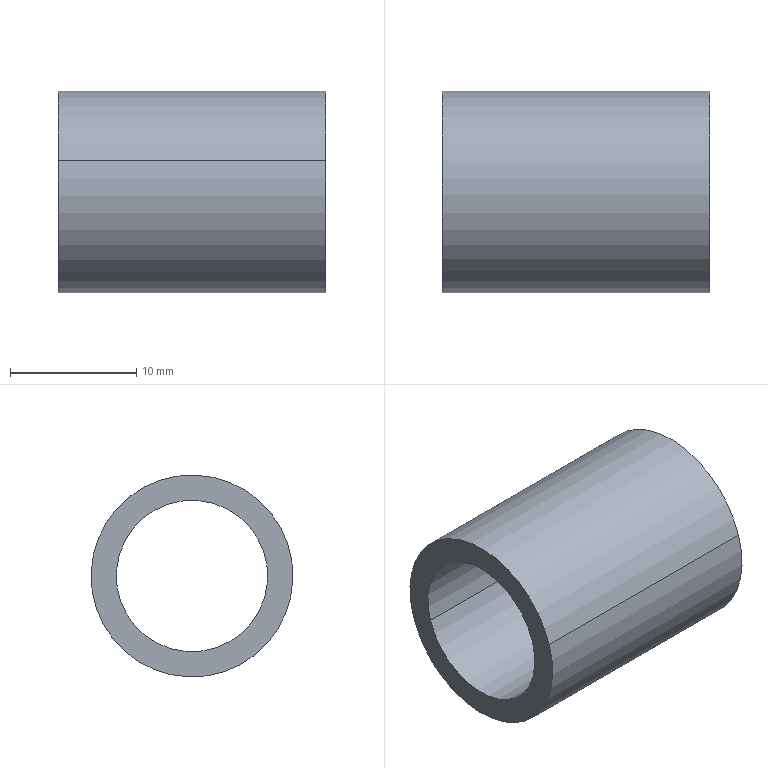Part | STEP file | Completa.sldasm-Part-4_Valor predeterminado | 1 solid | 6 faces | box 21.228 x 16 x 16 mm | volume 1867 mm3 | cylinder 4 | plane 2 | commonest cylinder face diameters 12 x2 16 x2
STEP:
#1=CARTESIAN_POINT('',(0.,0.,0.));
#2=DIRECTION('',(0.,0.,1.));
#3=DIRECTION('',(1.,0.,0.));
#4=AXIS2_PLACEMENT_3D('',#1,#2,#3);
#5=CARTESIAN_POINT('',(-204.167,20.156,-33.743));
#6=VERTEX_POINT('',#5);
#7=CARTESIAN_POINT('',(-225.395,20.156,-33.743));
#8=VERTEX_POINT('',#7);
#9=CARTESIAN_POINT('',(-204.167,20.156,-33.743));
#10=DIRECTION('',(-1.,0.,0.));
#11=VECTOR('',#10,1.);
#12=LINE('',#9,#11);
#13=CARTESIAN_POINT('',(-204.167,25.863,-35.597));
#14=DIRECTION('',(-1.,0.,0.));
#15=DIRECTION('',(0.,-0.9511,0.309));
#16=AXIS2_PLACEMENT_3D('',#13,#14,#15);
#17=CYLINDRICAL_SURFACE('',#16,6.);
#18=CARTESIAN_POINT('',(6.283,0.));
#19=DIRECTION('',(0.,1.));
#20=VECTOR('',#19,1.);
#21=LINE('',#18,#20);
#22=(GEOMETRIC_REPRESENTATION_CONTEXT(2)PARAMETRIC_REPRESENTATION_CONTEXT()REPRESENTATION_CONTEXT('',''));
#23=DEFINITIONAL_REPRESENTATION('',(#21),#22);
#24=PCURVE('',#17,#23);
#25=CARTESIAN_POINT('',(-204.167,25.863,-35.597));
#26=DIRECTION('',(-1.,0.,0.));
#27=DIRECTION('',(0.,-0.9511,0.309));
#28=AXIS2_PLACEMENT_3D('',#25,#26,#27);
#29=CYLINDRICAL_SURFACE('',#28,6.);
#30=CARTESIAN_POINT('',(0.,0.));
#31=DIRECTION('',(0.,1.));
#32=VECTOR('',#31,1.);
#33=LINE('',#30,#32);
#34=(GEOMETRIC_REPRESENTATION_CONTEXT(2)PARAMETRIC_REPRESENTATION_CONTEXT()REPRESENTATION_CONTEXT('',''));
#35=DEFINITIONAL_REPRESENTATION('',(#33),#34);
#36=PCURVE('',#29,#35);
#37=SURFACE_CURVE('',#12,(#24,#36),.PCURVE_S1.);
#38=EDGE_CURVE('',#6,#8,#37,.T.);
#39=ORIENTED_EDGE('',*,*,#38,.T.);
#40=CARTESIAN_POINT('',(-225.395,31.569,-37.451));
#41=VERTEX_POINT('',#40);
#42=CARTESIAN_POINT('',(-225.395,25.863,-35.597));
#43=DIRECTION('',(-1.,0.,0.));
#44=DIRECTION('',(0.,0.9511,-0.309));
#45=AXIS2_PLACEMENT_3D('',#42,#43,#44);
#46=CIRCLE('',#45,6.);
#47=CARTESIAN_POINT('',(3.142,21.228));
#48=DIRECTION('',(1.,0.));
#49=VECTOR('',#48,1.);
#50=LINE('',#47,#49);
#51=(GEOMETRIC_REPRESENTATION_CONTEXT(2)PARAMETRIC_REPRESENTATION_CONTEXT()REPRESENTATION_CONTEXT('',''));
#52=DEFINITIONAL_REPRESENTATION('',(#50),#51);
#53=PCURVE('',#17,#52);
#54=CARTESIAN_POINT('',(-225.395,-10.072,-30.999));
#55=DIRECTION('',(1.,0.,0.));
#56=DIRECTION('',(0.,0.9511,-0.309));
#57=AXIS2_PLACEMENT_3D('',#54,#55,#56);
#58=PLANE('',#57);
#59=CARTESIAN_POINT('',(41.597,6.731));
#60=CARTESIAN_POINT('',(41.597,-3.661));
#61=CARTESIAN_POINT('',(32.597,1.535));
#62=CARTESIAN_POINT('',(23.597,6.731));
#63=CARTESIAN_POINT('',(32.597,11.927));
#64=CARTESIAN_POINT('',(41.597,17.124));
#65=CARTESIAN_POINT('',(41.597,6.731));
#66=(BOUNDED_CURVE()B_SPLINE_CURVE(2,(#59,#60,#61,#62,#63,#64,#65),.UNSPECIFIED.,.T.,.F.)B_SPLINE_CURVE_WITH_KNOTS((1,2,2,2,2,1),(-2.094,0.,2.094,4.189,6.283,8.378),.UNSPECIFIED.)CURVE()GEOMETRIC_REPRESENTATION_ITEM()RATIONAL_B_SPLINE_CURVE((1.,0.5,1.,0.5,1.,0.5,1.))REPRESENTATION_ITEM(''));
#67=(GEOMETRIC_REPRESENTATION_CONTEXT(2)PARAMETRIC_REPRESENTATION_CONTEXT()REPRESENTATION_CONTEXT('',''));
#68=DEFINITIONAL_REPRESENTATION('',(#66),#67);
#69=PCURVE('',#58,#68);
#70=SURFACE_CURVE('',#46,(#53,#69),.PCURVE_S1.);
#71=EDGE_CURVE('',#41,#8,#70,.T.);
#72=ORIENTED_EDGE('',*,*,#71,.F.);
#73=CARTESIAN_POINT('',(-204.167,31.569,-37.451));
#74=VERTEX_POINT('',#73);
#75=CARTESIAN_POINT('',(-204.167,31.569,-37.451));
#76=DIRECTION('',(-1.,0.,0.));
#77=VECTOR('',#76,1.);
#78=LINE('',#75,#77);
#79=CARTESIAN_POINT('',(3.142,0.));
#80=DIRECTION('',(0.,1.));
#81=VECTOR('',#80,1.);
#82=LINE('',#79,#81);
#83=(GEOMETRIC_REPRESENTATION_CONTEXT(2)PARAMETRIC_REPRESENTATION_CONTEXT()REPRESENTATION_CONTEXT('',''));
#84=DEFINITIONAL_REPRESENTATION('',(#82),#83);
#85=PCURVE('',#17,#84);
#86=CARTESIAN_POINT('',(3.142,0.));
#87=DIRECTION('',(0.,1.));
#88=VECTOR('',#87,1.);
#89=LINE('',#86,#88);
#90=(GEOMETRIC_REPRESENTATION_CONTEXT(2)PARAMETRIC_REPRESENTATION_CONTEXT()REPRESENTATION_CONTEXT('',''));
#91=DEFINITIONAL_REPRESENTATION('',(#89),#90);
#92=PCURVE('',#29,#91);
#93=SURFACE_CURVE('',#78,(#85,#92),.PCURVE_S1.);
#94=EDGE_CURVE('',#74,#41,#93,.T.);
#95=ORIENTED_EDGE('',*,*,#94,.F.);
#96=CARTESIAN_POINT('',(-204.167,25.863,-35.597));
#97=DIRECTION('',(-1.,0.,0.));
#98=DIRECTION('',(0.,-0.9511,0.309));
#99=AXIS2_PLACEMENT_3D('',#96,#97,#98);
#100=CIRCLE('',#99,6.);
#101=CARTESIAN_POINT('',(0.,0.));
#102=DIRECTION('',(1.,0.));
#103=VECTOR('',#102,1.);
#104=LINE('',#101,#103);
#105=(GEOMETRIC_REPRESENTATION_CONTEXT(2)PARAMETRIC_REPRESENTATION_CONTEXT()REPRESENTATION_CONTEXT('',''));
#106=DEFINITIONAL_REPRESENTATION('',(#104),#105);
#107=PCURVE('',#17,#106);
#108=CARTESIAN_POINT('',(-204.167,25.863,-35.597));
#109=DIRECTION('',(1.,0.,0.));
#110=DIRECTION('',(0.,0.9511,-0.309));
#111=AXIS2_PLACEMENT_3D('',#108,#109,#110);
#112=PLANE('',#111);
#113=CARTESIAN_POINT('',(-6.,0.));
#114=CARTESIAN_POINT('',(-6.,10.392));
#115=CARTESIAN_POINT('',(3.,5.196));
#116=CARTESIAN_POINT('',(12.,0.));
#117=CARTESIAN_POINT('',(3.,-5.196));
#118=CARTESIAN_POINT('',(-6.,-10.392));
#119=CARTESIAN_POINT('',(-6.,0.));
#120=(BOUNDED_CURVE()B_SPLINE_CURVE(2,(#113,#114,#115,#116,#117,#118,#119),.UNSPECIFIED.,.T.,.F.)B_SPLINE_CURVE_WITH_KNOTS((1,2,2,2,2,1),(-2.094,0.,2.094,4.189,6.283,8.378),.UNSPECIFIED.)CURVE()GEOMETRIC_REPRESENTATION_ITEM()RATIONAL_B_SPLINE_CURVE((1.,0.5,1.,0.5,1.,0.5,1.))REPRESENTATION_ITEM(''));
#121=(GEOMETRIC_REPRESENTATION_CONTEXT(2)PARAMETRIC_REPRESENTATION_CONTEXT()REPRESENTATION_CONTEXT('',''));
#122=DEFINITIONAL_REPRESENTATION('',(#120),#121);
#123=PCURVE('',#112,#122);
#124=SURFACE_CURVE('',#100,(#107,#123),.PCURVE_S1.);
#125=EDGE_CURVE('',#74,#6,#124,.T.);
#126=ORIENTED_EDGE('',*,*,#125,.T.);
#127=EDGE_LOOP('',(#39,#72,#95,#126));
#128=FACE_BOUND('',#127,.F.);
#129=ADVANCED_FACE('',(#128),#17,.F.);
#130=CARTESIAN_POINT('',(-204.167,18.254,-33.125));
#131=VERTEX_POINT('',#130);
#132=CARTESIAN_POINT('',(-204.167,33.471,-38.069));
#133=VERTEX_POINT('',#132);
#134=CARTESIAN_POINT('',(-204.167,25.863,-35.597));
#135=DIRECTION('',(-1.,0.,0.));
#136=DIRECTION('',(0.,-0.9511,0.309));
#137=AXIS2_PLACEMENT_3D('',#134,#135,#136);
#138=CIRCLE('',#137,8.);
#139=CARTESIAN_POINT('',(-204.167,25.863,-35.597));
#140=DIRECTION('',(-1.,0.,0.));
#141=DIRECTION('',(0.,-0.9511,0.309));
#142=AXIS2_PLACEMENT_3D('',#139,#140,#141);
#143=CYLINDRICAL_SURFACE('',#142,8.);
#144=CARTESIAN_POINT('',(0.,0.));
#145=DIRECTION('',(1.,0.));
#146=VECTOR('',#145,1.);
#147=LINE('',#144,#146);
#148=(GEOMETRIC_REPRESENTATION_CONTEXT(2)PARAMETRIC_REPRESENTATION_CONTEXT()REPRESENTATION_CONTEXT('',''));
#149=DEFINITIONAL_REPRESENTATION('',(#147),#148);
#150=PCURVE('',#143,#149);
#151=CARTESIAN_POINT('',(-8.,0.));
#152=CARTESIAN_POINT('',(-8.,13.856));
#153=CARTESIAN_POINT('',(4.,6.928));
#154=CARTESIAN_POINT('',(16.,0.));
#155=CARTESIAN_POINT('',(4.,-6.928));
#156=CARTESIAN_POINT('',(-8.,-13.856));
#157=CARTESIAN_POINT('',(-8.,0.));
#158=(BOUNDED_CURVE()B_SPLINE_CURVE(2,(#151,#152,#153,#154,#155,#156,#157),.UNSPECIFIED.,.T.,.F.)B_SPLINE_CURVE_WITH_KNOTS((1,2,2,2,2,1),(-2.094,0.,2.094,4.189,6.283,8.378),.UNSPECIFIED.)CURVE()GEOMETRIC_REPRESENTATION_ITEM()RATIONAL_B_SPLINE_CURVE((1.,0.5,1.,0.5,1.,0.5,1.))REPRESENTATION_ITEM(''));
#159=(GEOMETRIC_REPRESENTATION_CONTEXT(2)PARAMETRIC_REPRESENTATION_CONTEXT()REPRESENTATION_CONTEXT('',''));
#160=DEFINITIONAL_REPRESENTATION('',(#158),#159);
#161=PCURVE('',#112,#160);
#162=SURFACE_CURVE('',#138,(#150,#161),.PCURVE_S1.);
#163=EDGE_CURVE('',#131,#133,#162,.T.);
#164=ORIENTED_EDGE('',*,*,#163,.T.);
#165=CARTESIAN_POINT('',(-225.395,33.471,-38.069));
#166=VERTEX_POINT('',#165);
#167=CARTESIAN_POINT('',(-204.167,33.471,-38.069));
#168=DIRECTION('',(-1.,0.,0.));
#169=VECTOR('',#168,1.);
#170=LINE('',#167,#169);
#171=CARTESIAN_POINT('',(3.142,0.));
#172=DIRECTION('',(0.,1.));
#173=VECTOR('',#172,1.);
#174=LINE('',#171,#173);
#175=(GEOMETRIC_REPRESENTATION_CONTEXT(2)PARAMETRIC_REPRESENTATION_CONTEXT()REPRESENTATION_CONTEXT('',''));
#176=DEFINITIONAL_REPRESENTATION('',(#174),#175);
#177=PCURVE('',#143,#176);
#178=CARTESIAN_POINT('',(-204.167,25.863,-35.597));
#179=DIRECTION('',(-1.,0.,0.));
#180=DIRECTION('',(0.,-0.9511,0.309));
#181=AXIS2_PLACEMENT_3D('',#178,#179,#180);
#182=CYLINDRICAL_SURFACE('',#181,8.);
#183=CARTESIAN_POINT('',(3.142,0.));
#184=DIRECTION('',(0.,1.));
#185=VECTOR('',#184,1.);
#186=LINE('',#183,#185);
#187=(GEOMETRIC_REPRESENTATION_CONTEXT(2)PARAMETRIC_REPRESENTATION_CONTEXT()REPRESENTATION_CONTEXT('',''));
#188=DEFINITIONAL_REPRESENTATION('',(#186),#187);
#189=PCURVE('',#182,#188);
#190=SURFACE_CURVE('',#170,(#177,#189),.PCURVE_S1.);
#191=EDGE_CURVE('',#133,#166,#190,.T.);
#192=ORIENTED_EDGE('',*,*,#191,.T.);
#193=CARTESIAN_POINT('',(-225.395,18.254,-33.125));
#194=VERTEX_POINT('',#193);
#195=CARTESIAN_POINT('',(-225.395,25.863,-35.597));
#196=DIRECTION('',(-1.,0.,0.));
#197=DIRECTION('',(0.,0.9511,-0.309));
#198=AXIS2_PLACEMENT_3D('',#195,#196,#197);
#199=CIRCLE('',#198,8.);
#200=CARTESIAN_POINT('',(-3.142,21.228));
#201=DIRECTION('',(1.,0.));
#202=VECTOR('',#201,1.);
#203=LINE('',#200,#202);
#204=(GEOMETRIC_REPRESENTATION_CONTEXT(2)PARAMETRIC_REPRESENTATION_CONTEXT()REPRESENTATION_CONTEXT('',''));
#205=DEFINITIONAL_REPRESENTATION('',(#203),#204);
#206=PCURVE('',#143,#205);
#207=CARTESIAN_POINT('',(43.597,6.731));
#208=CARTESIAN_POINT('',(43.597,-7.125));
#209=CARTESIAN_POINT('',(31.597,-0.1969));
#210=CARTESIAN_POINT('',(19.597,6.731));
#211=CARTESIAN_POINT('',(31.597,13.659));
#212=CARTESIAN_POINT('',(43.597,20.588));
#213=CARTESIAN_POINT('',(43.597,6.731));
#214=(BOUNDED_CURVE()B_SPLINE_CURVE(2,(#207,#208,#209,#210,#211,#212,#213),.UNSPECIFIED.,.T.,.F.)B_SPLINE_CURVE_WITH_KNOTS((1,2,2,2,2,1),(-2.094,0.,2.094,4.189,6.283,8.378),.UNSPECIFIED.)CURVE()GEOMETRIC_REPRESENTATION_ITEM()RATIONAL_B_SPLINE_CURVE((1.,0.5,1.,0.5,1.,0.5,1.))REPRESENTATION_ITEM(''));
#215=(GEOMETRIC_REPRESENTATION_CONTEXT(2)PARAMETRIC_REPRESENTATION_CONTEXT()REPRESENTATION_CONTEXT('',''));
#216=DEFINITIONAL_REPRESENTATION('',(#214),#215);
#217=PCURVE('',#58,#216);
#218=SURFACE_CURVE('',#199,(#206,#217),.PCURVE_S1.);
#219=EDGE_CURVE('',#194,#166,#218,.T.);
#220=ORIENTED_EDGE('',*,*,#219,.F.);
#221=CARTESIAN_POINT('',(-204.167,18.254,-33.125));
#222=DIRECTION('',(-1.,0.,0.));
#223=VECTOR('',#222,1.);
#224=LINE('',#221,#223);
#225=CARTESIAN_POINT('',(0.,0.));
#226=DIRECTION('',(0.,1.));
#227=VECTOR('',#226,1.);
#228=LINE('',#225,#227);
#229=(GEOMETRIC_REPRESENTATION_CONTEXT(2)PARAMETRIC_REPRESENTATION_CONTEXT()REPRESENTATION_CONTEXT('',''));
#230=DEFINITIONAL_REPRESENTATION('',(#228),#229);
#231=PCURVE('',#143,#230);
#232=CARTESIAN_POINT('',(6.283,0.));
#233=DIRECTION('',(0.,1.));
#234=VECTOR('',#233,1.);
#235=LINE('',#232,#234);
#236=(GEOMETRIC_REPRESENTATION_CONTEXT(2)PARAMETRIC_REPRESENTATION_CONTEXT()REPRESENTATION_CONTEXT('',''));
#237=DEFINITIONAL_REPRESENTATION('',(#235),#236);
#238=PCURVE('',#182,#237);
#239=SURFACE_CURVE('',#224,(#231,#238),.PCURVE_S1.);
#240=EDGE_CURVE('',#131,#194,#239,.T.);
#241=ORIENTED_EDGE('',*,*,#240,.F.);
#242=EDGE_LOOP('',(#164,#192,#220,#241));
#243=FACE_BOUND('',#242,.T.);
#244=ADVANCED_FACE('',(#243),#143,.T.);
#245=ORIENTED_EDGE('',*,*,#191,.F.);
#246=CARTESIAN_POINT('',(-204.167,25.863,-35.597));
#247=DIRECTION('',(-1.,0.,0.));
#248=DIRECTION('',(0.,-0.9511,0.309));
#249=AXIS2_PLACEMENT_3D('',#246,#247,#248);
#250=CIRCLE('',#249,8.);
#251=CARTESIAN_POINT('',(0.,0.));
#252=DIRECTION('',(1.,0.));
#253=VECTOR('',#252,1.);
#254=LINE('',#251,#253);
#255=(GEOMETRIC_REPRESENTATION_CONTEXT(2)PARAMETRIC_REPRESENTATION_CONTEXT()REPRESENTATION_CONTEXT('',''));
#256=DEFINITIONAL_REPRESENTATION('',(#254),#255);
#257=PCURVE('',#182,#256);
#258=CARTESIAN_POINT('',(-8.,0.));
#259=CARTESIAN_POINT('',(-8.,13.856));
#260=CARTESIAN_POINT('',(4.,6.928));
#261=CARTESIAN_POINT('',(16.,0.));
#262=CARTESIAN_POINT('',(4.,-6.928));
#263=CARTESIAN_POINT('',(-8.,-13.856));
#264=CARTESIAN_POINT('',(-8.,0.));
#265=(BOUNDED_CURVE()B_SPLINE_CURVE(2,(#258,#259,#260,#261,#262,#263,#264),.UNSPECIFIED.,.T.,.F.)B_SPLINE_CURVE_WITH_KNOTS((1,2,2,2,2,1),(-2.094,0.,2.094,4.189,6.283,8.378),.UNSPECIFIED.)CURVE()GEOMETRIC_REPRESENTATION_ITEM()RATIONAL_B_SPLINE_CURVE((1.,0.5,1.,0.5,1.,0.5,1.))REPRESENTATION_ITEM(''));
#266=(GEOMETRIC_REPRESENTATION_CONTEXT(2)PARAMETRIC_REPRESENTATION_CONTEXT()REPRESENTATION_CONTEXT('',''));
#267=DEFINITIONAL_REPRESENTATION('',(#265),#266);
#268=PCURVE('',#112,#267);
#269=SURFACE_CURVE('',#250,(#257,#268),.PCURVE_S1.);
#270=EDGE_CURVE('',#133,#131,#269,.T.);
#271=ORIENTED_EDGE('',*,*,#270,.T.);
#272=ORIENTED_EDGE('',*,*,#240,.T.);
#273=CARTESIAN_POINT('',(-225.395,25.863,-35.597));
#274=DIRECTION('',(-1.,0.,0.));
#275=DIRECTION('',(0.,0.9511,-0.309));
#276=AXIS2_PLACEMENT_3D('',#273,#274,#275);
#277=CIRCLE('',#276,8.);
#278=CARTESIAN_POINT('',(3.142,21.228));
#279=DIRECTION('',(1.,0.));
#280=VECTOR('',#279,1.);
#281=LINE('',#278,#280);
#282=(GEOMETRIC_REPRESENTATION_CONTEXT(2)PARAMETRIC_REPRESENTATION_CONTEXT()REPRESENTATION_CONTEXT('',''));
#283=DEFINITIONAL_REPRESENTATION('',(#281),#282);
#284=PCURVE('',#182,#283);
#285=CARTESIAN_POINT('',(43.597,6.731));
#286=CARTESIAN_POINT('',(43.597,-7.125));
#287=CARTESIAN_POINT('',(31.597,-0.1969));
#288=CARTESIAN_POINT('',(19.597,6.731));
#289=CARTESIAN_POINT('',(31.597,13.659));
#290=CARTESIAN_POINT('',(43.597,20.588));
#291=CARTESIAN_POINT('',(43.597,6.731));
#292=(BOUNDED_CURVE()B_SPLINE_CURVE(2,(#285,#286,#287,#288,#289,#290,#291),.UNSPECIFIED.,.T.,.F.)B_SPLINE_CURVE_WITH_KNOTS((1,2,2,2,2,1),(-2.094,0.,2.094,4.189,6.283,8.378),.UNSPECIFIED.)CURVE()GEOMETRIC_REPRESENTATION_ITEM()RATIONAL_B_SPLINE_CURVE((1.,0.5,1.,0.5,1.,0.5,1.))REPRESENTATION_ITEM(''));
#293=(GEOMETRIC_REPRESENTATION_CONTEXT(2)PARAMETRIC_REPRESENTATION_CONTEXT()REPRESENTATION_CONTEXT('',''));
#294=DEFINITIONAL_REPRESENTATION('',(#292),#293);
#295=PCURVE('',#58,#294);
#296=SURFACE_CURVE('',#277,(#284,#295),.PCURVE_S1.);
#297=EDGE_CURVE('',#166,#194,#296,.T.);
#298=ORIENTED_EDGE('',*,*,#297,.F.);
#299=EDGE_LOOP('',(#245,#271,#272,#298));
#300=FACE_BOUND('',#299,.T.);
#301=ADVANCED_FACE('',(#300),#182,.T.);
#302=ORIENTED_EDGE('',*,*,#163,.F.);
#303=ORIENTED_EDGE('',*,*,#270,.F.);
#304=EDGE_LOOP('',(#302,#303));
#305=FACE_BOUND('',#304,.T.);
#306=CARTESIAN_POINT('',(-204.167,25.863,-35.597));
#307=DIRECTION('',(-1.,0.,0.));
#308=DIRECTION('',(0.,-0.9511,0.309));
#309=AXIS2_PLACEMENT_3D('',#306,#307,#308);
#310=CIRCLE('',#309,6.);
#311=CARTESIAN_POINT('',(-6.,0.));
#312=CARTESIAN_POINT('',(-6.,10.392));
#313=CARTESIAN_POINT('',(3.,5.196));
#314=CARTESIAN_POINT('',(12.,0.));
#315=CARTESIAN_POINT('',(3.,-5.196));
#316=CARTESIAN_POINT('',(-6.,-10.392));
#317=CARTESIAN_POINT('',(-6.,0.));
#318=(BOUNDED_CURVE()B_SPLINE_CURVE(2,(#311,#312,#313,#314,#315,#316,#317),.UNSPECIFIED.,.T.,.F.)B_SPLINE_CURVE_WITH_KNOTS((1,2,2,2,2,1),(-2.094,0.,2.094,4.189,6.283,8.378),.UNSPECIFIED.)CURVE()GEOMETRIC_REPRESENTATION_ITEM()RATIONAL_B_SPLINE_CURVE((1.,0.5,1.,0.5,1.,0.5,1.))REPRESENTATION_ITEM(''));
#319=(GEOMETRIC_REPRESENTATION_CONTEXT(2)PARAMETRIC_REPRESENTATION_CONTEXT()REPRESENTATION_CONTEXT('',''));
#320=DEFINITIONAL_REPRESENTATION('',(#318),#319);
#321=PCURVE('',#112,#320);
#322=CARTESIAN_POINT('',(0.,0.));
#323=DIRECTION('',(1.,0.));
#324=VECTOR('',#323,1.);
#325=LINE('',#322,#324);
#326=(GEOMETRIC_REPRESENTATION_CONTEXT(2)PARAMETRIC_REPRESENTATION_CONTEXT()REPRESENTATION_CONTEXT('',''));
#327=DEFINITIONAL_REPRESENTATION('',(#325),#326);
#328=PCURVE('',#29,#327);
#329=SURFACE_CURVE('',#310,(#321,#328),.PCURVE_S1.);
#330=EDGE_CURVE('',#6,#74,#329,.T.);
#331=ORIENTED_EDGE('',*,*,#330,.T.);
#332=ORIENTED_EDGE('',*,*,#125,.T.);
#333=EDGE_LOOP('',(#331,#332));
#334=FACE_BOUND('',#333,.T.);
#335=ADVANCED_FACE('',(#305,#334),#112,.T.);
#336=CARTESIAN_POINT('',(-225.395,25.863,-35.597));
#337=DIRECTION('',(-1.,0.,0.));
#338=DIRECTION('',(0.,0.9511,-0.309));
#339=AXIS2_PLACEMENT_3D('',#336,#337,#338);
#340=CIRCLE('',#339,6.);
#341=CARTESIAN_POINT('',(-3.142,21.228));
#342=DIRECTION('',(1.,0.));
#343=VECTOR('',#342,1.);
#344=LINE('',#341,#343);
#345=(GEOMETRIC_REPRESENTATION_CONTEXT(2)PARAMETRIC_REPRESENTATION_CONTEXT()REPRESENTATION_CONTEXT('',''));
#346=DEFINITIONAL_REPRESENTATION('',(#344),#345);
#347=PCURVE('',#29,#346);
#348=CARTESIAN_POINT('',(41.597,6.731));
#349=CARTESIAN_POINT('',(41.597,-3.661));
#350=CARTESIAN_POINT('',(32.597,1.535));
#351=CARTESIAN_POINT('',(23.597,6.731));
#352=CARTESIAN_POINT('',(32.597,11.927));
#353=CARTESIAN_POINT('',(41.597,17.124));
#354=CARTESIAN_POINT('',(41.597,6.731));
#355=(BOUNDED_CURVE()B_SPLINE_CURVE(2,(#348,#349,#350,#351,#352,#353,#354),.UNSPECIFIED.,.T.,.F.)B_SPLINE_CURVE_WITH_KNOTS((1,2,2,2,2,1),(-2.094,0.,2.094,4.189,6.283,8.378),.UNSPECIFIED.)CURVE()GEOMETRIC_REPRESENTATION_ITEM()RATIONAL_B_SPLINE_CURVE((1.,0.5,1.,0.5,1.,0.5,1.))REPRESENTATION_ITEM(''));
#356=(GEOMETRIC_REPRESENTATION_CONTEXT(2)PARAMETRIC_REPRESENTATION_CONTEXT()REPRESENTATION_CONTEXT('',''));
#357=DEFINITIONAL_REPRESENTATION('',(#355),#356);
#358=PCURVE('',#58,#357);
#359=SURFACE_CURVE('',#340,(#347,#358),.PCURVE_S1.);
#360=EDGE_CURVE('',#8,#41,#359,.T.);
#361=ORIENTED_EDGE('',*,*,#360,.F.);
#362=ORIENTED_EDGE('',*,*,#38,.F.);
#363=ORIENTED_EDGE('',*,*,#330,.T.);
#364=ORIENTED_EDGE('',*,*,#94,.T.);
#365=EDGE_LOOP('',(#361,#362,#363,#364));
#366=FACE_BOUND('',#365,.F.);
#367=ADVANCED_FACE('',(#366),#29,.F.);
#368=ORIENTED_EDGE('',*,*,#219,.T.);
#369=ORIENTED_EDGE('',*,*,#297,.T.);
#370=EDGE_LOOP('',(#368,#369));
#371=FACE_BOUND('',#370,.T.);
#372=ORIENTED_EDGE('',*,*,#360,.F.);
#373=ORIENTED_EDGE('',*,*,#71,.F.);
#374=EDGE_LOOP('',(#372,#373));
#375=FACE_BOUND('',#374,.T.);
#376=ADVANCED_FACE('',(#371,#375),#58,.F.);
#377=CLOSED_SHELL('',(#129,#244,#301,#335,#367,#376));
#378=MANIFOLD_SOLID_BREP('',#377);
#379=(LENGTH_UNIT()NAMED_UNIT(*)SI_UNIT(.MILLI.,.METRE.));
#380=UNCERTAINTY_MEASURE_WITH_UNIT(LENGTH_MEASURE(0.0000001),#379,'','');
#381=(NAMED_UNIT(*)PLANE_ANGLE_UNIT()SI_UNIT($,.RADIAN.));
#382=(NAMED_UNIT(*)SI_UNIT($,.STERADIAN.)SOLID_ANGLE_UNIT());
#383=(GEOMETRIC_REPRESENTATION_CONTEXT(3)GLOBAL_UNCERTAINTY_ASSIGNED_CONTEXT((#380))GLOBAL_UNIT_ASSIGNED_CONTEXT((#379,#381,#382))REPRESENTATION_CONTEXT('',''));
#384=ADVANCED_BREP_SHAPE_REPRESENTATION('',(#4,#378),#383);